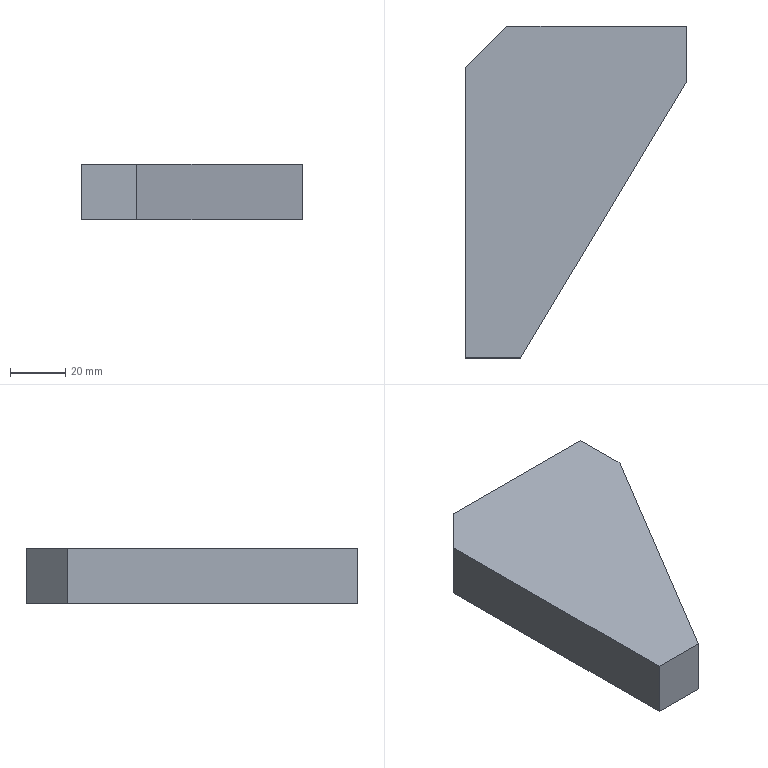Part | SolidWorks | features Extrusion 1 | 1 solid | 8 faces | box 80 x 120 x 20 mm | volume 129750 mm3 | plane 8
STEP:
#1=CARTESIAN_POINT('',(0.,0.,0.));
#2=VERTEX_POINT('',#1);
#3=CARTESIAN_POINT('',(20.,0.,0.));
#4=VERTEX_POINT('',#3);
#5=CARTESIAN_POINT('',(20.,0.,0.));
#6=DIRECTION('',(1.,0.,0.));
#7=VECTOR('',#6,1000.);
#8=LINE('',#5,#7);
#9=EDGE_CURVE('',#2,#4,#8,.T.);
#10=ORIENTED_EDGE('',*,*,#9,.T.);
#11=CARTESIAN_POINT('',(20.,0.,20.));
#12=VERTEX_POINT('',#11);
#13=CARTESIAN_POINT('',(20.,0.,20.));
#14=DIRECTION('',(0.,0.,-1.));
#15=VECTOR('',#14,1000.);
#16=LINE('',#13,#15);
#17=EDGE_CURVE('',#12,#4,#16,.T.);
#18=ORIENTED_EDGE('',*,*,#17,.F.);
#19=CARTESIAN_POINT('',(0.,0.,20.));
#20=VERTEX_POINT('',#19);
#21=CARTESIAN_POINT('',(20.,0.,20.));
#22=DIRECTION('',(1.,0.,0.));
#23=VECTOR('',#22,1000.);
#24=LINE('',#21,#23);
#25=EDGE_CURVE('',#20,#12,#24,.T.);
#26=ORIENTED_EDGE('',*,*,#25,.F.);
#27=CARTESIAN_POINT('',(0.,0.,20.));
#28=DIRECTION('',(0.,0.,-1.));
#29=VECTOR('',#28,1000.);
#30=LINE('',#27,#29);
#31=EDGE_CURVE('',#20,#2,#30,.T.);
#32=ORIENTED_EDGE('',*,*,#31,.T.);
#33=EDGE_LOOP('',(#10,#18,#26,#32));
#34=FACE_OUTER_BOUND('',#33,.T.);
#35=CARTESIAN_POINT('',(20.,0.,20.));
#36=DIRECTION('',(0.,1.,0.));
#37=DIRECTION('',(-1.,0.,0.));
#38=AXIS2_PLACEMENT_3D('',#35,#36,#37);
#39=PLANE('',#38);
#40=ADVANCED_FACE('',(#34),#39,.F.);
#41=CARTESIAN_POINT('',(80.,100.,0.));
#42=VERTEX_POINT('',#41);
#43=CARTESIAN_POINT('',(80.,100.,0.));
#44=DIRECTION('',(0.5145,0.8575,0.));
#45=VECTOR('',#44,1000.);
#46=LINE('',#43,#45);
#47=EDGE_CURVE('',#4,#42,#46,.T.);
#48=ORIENTED_EDGE('',*,*,#47,.T.);
#49=CARTESIAN_POINT('',(80.,100.,20.));
#50=VERTEX_POINT('',#49);
#51=CARTESIAN_POINT('',(80.,100.,20.));
#52=DIRECTION('',(0.,0.,-1.));
#53=VECTOR('',#52,1000.);
#54=LINE('',#51,#53);
#55=EDGE_CURVE('',#50,#42,#54,.T.);
#56=ORIENTED_EDGE('',*,*,#55,.F.);
#57=CARTESIAN_POINT('',(80.,100.,20.));
#58=DIRECTION('',(0.5145,0.8575,0.));
#59=VECTOR('',#58,1000.);
#60=LINE('',#57,#59);
#61=EDGE_CURVE('',#12,#50,#60,.T.);
#62=ORIENTED_EDGE('',*,*,#61,.F.);
#63=ORIENTED_EDGE('',*,*,#17,.T.);
#64=EDGE_LOOP('',(#48,#56,#62,#63));
#65=FACE_OUTER_BOUND('',#64,.T.);
#66=CARTESIAN_POINT('',(80.,100.,20.));
#67=DIRECTION('',(-0.8575,0.5145,0.));
#68=DIRECTION('',(-0.5145,-0.8575,0.));
#69=AXIS2_PLACEMENT_3D('',#66,#67,#68);
#70=PLANE('',#69);
#71=ADVANCED_FACE('',(#65),#70,.F.);
#72=CARTESIAN_POINT('',(80.,120.,0.));
#73=VERTEX_POINT('',#72);
#74=CARTESIAN_POINT('',(80.,120.,0.));
#75=DIRECTION('',(0.,1.,0.));
#76=VECTOR('',#75,1000.);
#77=LINE('',#74,#76);
#78=EDGE_CURVE('',#42,#73,#77,.T.);
#79=ORIENTED_EDGE('',*,*,#78,.T.);
#80=CARTESIAN_POINT('',(80.,120.,20.));
#81=VERTEX_POINT('',#80);
#82=CARTESIAN_POINT('',(80.,120.,20.));
#83=DIRECTION('',(0.,0.,-1.));
#84=VECTOR('',#83,1000.);
#85=LINE('',#82,#84);
#86=EDGE_CURVE('',#81,#73,#85,.T.);
#87=ORIENTED_EDGE('',*,*,#86,.F.);
#88=CARTESIAN_POINT('',(80.,120.,20.));
#89=DIRECTION('',(0.,1.,0.));
#90=VECTOR('',#89,1000.);
#91=LINE('',#88,#90);
#92=EDGE_CURVE('',#50,#81,#91,.T.);
#93=ORIENTED_EDGE('',*,*,#92,.F.);
#94=ORIENTED_EDGE('',*,*,#55,.T.);
#95=EDGE_LOOP('',(#79,#87,#93,#94));
#96=FACE_OUTER_BOUND('',#95,.T.);
#97=CARTESIAN_POINT('',(80.,120.,20.));
#98=DIRECTION('',(-1.,0.,0.));
#99=DIRECTION('',(0.,0.,1.));
#100=AXIS2_PLACEMENT_3D('',#97,#98,#99);
#101=PLANE('',#100);
#102=ADVANCED_FACE('',(#96),#101,.F.);
#103=CARTESIAN_POINT('',(15.,120.,0.));
#104=VERTEX_POINT('',#103);
#105=CARTESIAN_POINT('',(15.,120.,0.));
#106=DIRECTION('',(-1.,0.,0.));
#107=VECTOR('',#106,1000.);
#108=LINE('',#105,#107);
#109=EDGE_CURVE('',#73,#104,#108,.T.);
#110=ORIENTED_EDGE('',*,*,#109,.T.);
#111=CARTESIAN_POINT('',(15.,120.,20.));
#112=VERTEX_POINT('',#111);
#113=CARTESIAN_POINT('',(15.,120.,20.));
#114=DIRECTION('',(0.,0.,-1.));
#115=VECTOR('',#114,1000.);
#116=LINE('',#113,#115);
#117=EDGE_CURVE('',#112,#104,#116,.T.);
#118=ORIENTED_EDGE('',*,*,#117,.F.);
#119=CARTESIAN_POINT('',(15.,120.,20.));
#120=DIRECTION('',(-1.,0.,0.));
#121=VECTOR('',#120,1000.);
#122=LINE('',#119,#121);
#123=EDGE_CURVE('',#81,#112,#122,.T.);
#124=ORIENTED_EDGE('',*,*,#123,.F.);
#125=ORIENTED_EDGE('',*,*,#86,.T.);
#126=EDGE_LOOP('',(#110,#118,#124,#125));
#127=FACE_OUTER_BOUND('',#126,.T.);
#128=CARTESIAN_POINT('',(15.,120.,20.));
#129=DIRECTION('',(0.,-1.,0.));
#130=DIRECTION('',(0.,0.,-1.));
#131=AXIS2_PLACEMENT_3D('',#128,#129,#130);
#132=PLANE('',#131);
#133=ADVANCED_FACE('',(#127),#132,.F.);
#134=CARTESIAN_POINT('',(0.,105.,0.));
#135=VERTEX_POINT('',#134);
#136=CARTESIAN_POINT('',(0.,105.,0.));
#137=DIRECTION('',(-0.7071,-0.7071,0.));
#138=VECTOR('',#137,1000.);
#139=LINE('',#136,#138);
#140=EDGE_CURVE('',#104,#135,#139,.T.);
#141=ORIENTED_EDGE('',*,*,#140,.T.);
#142=CARTESIAN_POINT('',(0.,105.,20.));
#143=VERTEX_POINT('',#142);
#144=CARTESIAN_POINT('',(0.,105.,20.));
#145=DIRECTION('',(0.,0.,-1.));
#146=VECTOR('',#145,1000.);
#147=LINE('',#144,#146);
#148=EDGE_CURVE('',#143,#135,#147,.T.);
#149=ORIENTED_EDGE('',*,*,#148,.F.);
#150=CARTESIAN_POINT('',(0.,105.,20.));
#151=DIRECTION('',(-0.7071,-0.7071,0.));
#152=VECTOR('',#151,1000.);
#153=LINE('',#150,#152);
#154=EDGE_CURVE('',#112,#143,#153,.T.);
#155=ORIENTED_EDGE('',*,*,#154,.F.);
#156=ORIENTED_EDGE('',*,*,#117,.T.);
#157=EDGE_LOOP('',(#141,#149,#155,#156));
#158=FACE_OUTER_BOUND('',#157,.T.);
#159=CARTESIAN_POINT('',(0.,105.,20.));
#160=DIRECTION('',(0.7071,-0.7071,0.));
#161=DIRECTION('',(0.7071,0.7071,0.));
#162=AXIS2_PLACEMENT_3D('',#159,#160,#161);
#163=PLANE('',#162);
#164=ADVANCED_FACE('',(#158),#163,.F.);
#165=CARTESIAN_POINT('',(0.,0.,0.));
#166=DIRECTION('',(0.,-1.,0.));
#167=VECTOR('',#166,1000.);
#168=LINE('',#165,#167);
#169=EDGE_CURVE('',#135,#2,#168,.T.);
#170=ORIENTED_EDGE('',*,*,#169,.T.);
#171=ORIENTED_EDGE('',*,*,#31,.F.);
#172=CARTESIAN_POINT('',(0.,0.,20.));
#173=DIRECTION('',(0.,-1.,0.));
#174=VECTOR('',#173,1000.);
#175=LINE('',#172,#174);
#176=EDGE_CURVE('',#143,#20,#175,.T.);
#177=ORIENTED_EDGE('',*,*,#176,.F.);
#178=ORIENTED_EDGE('',*,*,#148,.T.);
#179=EDGE_LOOP('',(#170,#171,#177,#178));
#180=FACE_OUTER_BOUND('',#179,.T.);
#181=CARTESIAN_POINT('',(0.,0.,20.));
#182=DIRECTION('',(1.,0.,0.));
#183=DIRECTION('',(0.,0.,-1.));
#184=AXIS2_PLACEMENT_3D('',#181,#182,#183);
#185=PLANE('',#184);
#186=ADVANCED_FACE('',(#180),#185,.F.);
#187=ORIENTED_EDGE('',*,*,#25,.T.);
#188=ORIENTED_EDGE('',*,*,#61,.T.);
#189=ORIENTED_EDGE('',*,*,#92,.T.);
#190=ORIENTED_EDGE('',*,*,#123,.T.);
#191=ORIENTED_EDGE('',*,*,#154,.T.);
#192=ORIENTED_EDGE('',*,*,#176,.T.);
#193=EDGE_LOOP('',(#187,#188,#189,#190,#191,#192));
#194=FACE_OUTER_BOUND('',#193,.T.);
#195=CARTESIAN_POINT('',(0.,0.,20.));
#196=DIRECTION('',(0.,0.,-1.));
#197=DIRECTION('',(-1.,0.,0.));
#198=AXIS2_PLACEMENT_3D('',#195,#196,#197);
#199=PLANE('',#198);
#200=ADVANCED_FACE('',(#194),#199,.F.);
#201=ORIENTED_EDGE('',*,*,#9,.F.);
#202=ORIENTED_EDGE('',*,*,#169,.F.);
#203=ORIENTED_EDGE('',*,*,#140,.F.);
#204=ORIENTED_EDGE('',*,*,#109,.F.);
#205=ORIENTED_EDGE('',*,*,#78,.F.);
#206=ORIENTED_EDGE('',*,*,#47,.F.);
#207=EDGE_LOOP('',(#201,#202,#203,#204,#205,#206));
#208=FACE_OUTER_BOUND('',#207,.T.);
#209=CARTESIAN_POINT('',(0.,0.,0.));
#210=DIRECTION('',(0.,0.,-1.));
#211=DIRECTION('',(-1.,0.,0.));
#212=AXIS2_PLACEMENT_3D('',#209,#210,#211);
#213=PLANE('',#212);
#214=ADVANCED_FACE('',(#208),#213,.T.);
#215=CLOSED_SHELL('',(#40,#71,#102,#133,#164,#186,#200,#214));
#216=MANIFOLD_SOLID_BREP('',#215);
#217=CARTESIAN_POINT('',(0.,0.,0.));
#218=DIRECTION('',(0.,0.,1.));
#219=DIRECTION('',(1.,0.,0.));
#220=AXIS2_PLACEMENT_3D('',#217,#218,#219);
#221=(LENGTH_UNIT()NAMED_UNIT(*)SI_UNIT(.MILLI.,.METRE.));
#222=UNCERTAINTY_MEASURE_WITH_UNIT(LENGTH_MEASURE(0.00001),#221,'','');
#223=(NAMED_UNIT(*)PLANE_ANGLE_UNIT()SI_UNIT($,.RADIAN.));
#224=(NAMED_UNIT(*)SI_UNIT($,.STERADIAN.)SOLID_ANGLE_UNIT());
#225=(GEOMETRIC_REPRESENTATION_CONTEXT(3)GLOBAL_UNCERTAINTY_ASSIGNED_CONTEXT((#222))GLOBAL_UNIT_ASSIGNED_CONTEXT((#221,#223,#224))REPRESENTATION_CONTEXT('',''));
#226=ADVANCED_BREP_SHAPE_REPRESENTATION('',(#216,#220),#225);